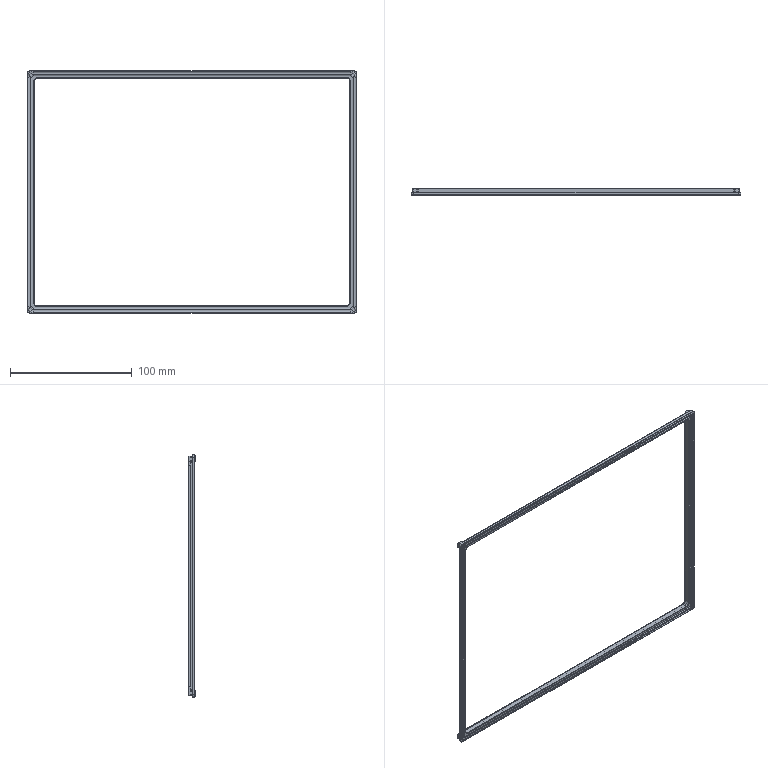Part | SolidWorks | features BaseBody 1 | 1 solid | 179 faces | box 270.8 x 5.7 x 198.8 mm | volume 17493 mm3 | plane 83 | cylinder 60 | cone 20 | spline 16 | commonest cylinder face diameters 1 x28 0.6 x16 4 x4 6 x4 7.8 x4 9.8 x4